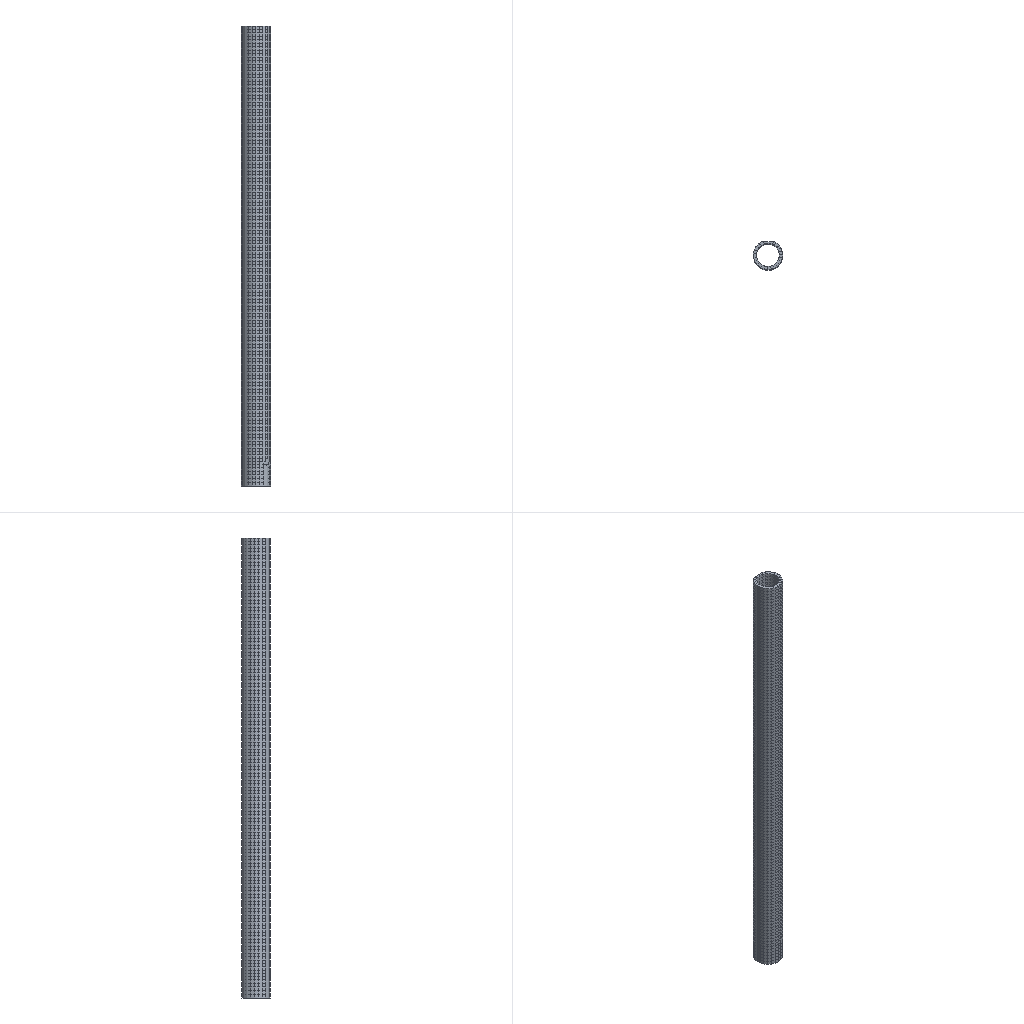Simulation study | abaqus
Set-up summary:
category,name,step,type,value,unit,region
solver,abaqus,,Abaqus/CAE 2024
units,mm-N-s-tonne (MPa),,inferred,E=210000 density=
analysis,Step-4,,static,time_period=10
mesh,nodes,,,6433
mesh,elements,,,3192
element_type,C3D8R,,,3192
material,Material-1,,E,210000
material,Material-1,,nu,0.3
material,Material-1,,yield,380
material,Material-1,,cte,1.3e-05
material,Material-1,,behaviors,plastic; expansion
section,Material-1,,solid section,,,Set-1
load,Load-2,Step-4,pressure,30,,Surf-6
load,Load-4,Step-4,concentrated force,"1000 [dir=(0, 1, 0)]",,Set-13
bc,BC-1,initial,fixed,"[dofs=rx,ry,rz,x,y,z n=6]",,Set-5
bc,BC-2,Step-4,displacement,-0.5 [dofs=rx],,_PickedSet34
bc,BC-2,Step-4,fixed,"[dofs=ry,rz n=2]",,_PickedSet34
constraint,coupling,,,1
Abaqus input file, long lists of numbers shortened:
*Heading
** Job name: deck Model name: Model-1-3
** Generated by: Abaqus/CAE 2024
*Preprint, echo=NO, model=NO, history=NO, contact=NO
**
** PARTS
**
*Part, name=Part-10
*Node
      1,           0.,          58.,         120.
      2,           0.,          50.,         120.
** (6430 more lines like these left out)
*Element, type=C3D8R
   1,    1,    2,   33,    5,   54,  301,  973,  549
   2,    5,   33,   34,   47,  549,  973,  974, 2471
** (3190 more lines like these left out)
*Nset, nset=Set-1, generate
    1,  6432,     1
*Elset, elset=Set-1, generate
    1,  3192,     1
** Section: Section-1
*Solid Section, elset=Set-1, material=Material-1
,
*End Part
**
**
** ASSEMBLY
**
*Assembly, name=Assembly
**
*Instance, name=Part-10-1, part=Part-10
*End Instance
**
*Node
      1,           0., -3.91886993e-15,        2000.
*Nset, nset=Set-5, instance=Part-10-1
  22,  23,  24,  25,  26,  30,  31,  32, 906, 907, 908, 909, 910, 911, 912, 913
 914, 915, 916, 917, 918, 919, 920, 921, 922, 923, 924, 952, 953, 954, 955, 956
** (1 more lines like these left out)
*Elset, elset=Set-5, instance=Part-10-1
 3078, 3079, 3080, 3081, 3082, 3083, 3084, 3085, 3086, 3087, 3088, 3180, 3181, 3182, 3183, 3184
 3185, 3186, 3187, 3188, 3189, 3190, 3191, 3192
*Nset, nset=Set-13
 1,
*Nset, nset=m_Set-12
 1,
*Nset, nset=s_Set-8, instance=Part-10-1
   8,   9,  10,  11,  12,  13,  14,  16, 674, 675, 676, 677, 678, 679, 680, 681
 682, 683, 684, 685, 686, 687, 688, 689, 690, 691, 692, 693, 694, 838, 839, 840
** (1 more lines like these left out)
*Elset, elset=s_Set-8, instance=Part-10-1
 1613, 1614, 1615, 1616, 1617, 1618, 1619, 1620, 1621, 1622, 1623, 1624, 1625, 2990, 2991, 2992
 2993, 2994, 2995, 2996, 2997, 2998, 2999, 3000
*Nset, nset=_PickedSet34, internal
 1,
*Elset, elset=_Surf-2_S3, internal, instance=Part-10-1, generate
 3001,  3088,     1
*Elset, elset=_Surf-2_S5, internal, instance=Part-10-1, generate
 3089,  3192,     1
*Elset, elset=_Surf-2_S4, internal, instance=Part-10-1, generate
    1,  1625,     1
*Elset, elset=_Surf-2_S6, internal, instance=Part-10-1, generate
 1626,  3000,     1
*Surface, type=ELEMENT, name=Surf-2
_Surf-2_S3, S3
_Surf-2_S5, S5
_Surf-2_S4, S4
_Surf-2_S6, S6
*Elset, elset=_Surf-5_S5, internal, instance=Part-10-1
 3035, 3036, 3037, 3038, 3039, 3040, 3041, 3042, 3043, 3044, 3046, 3047, 3048, 3049, 3050, 3051
 3052, 3053, 3054, 3055, 3057, 3058, 3059, 3060, 3061, 3062, 3063, 3064, 3065, 3066, 3068, 3069
** (2 more lines like these left out)
*Elset, elset=_Surf-5_S3, internal, instance=Part-10-1
 3129, 3130, 3131, 3132, 3133, 3134, 3135, 3136, 3137, 3138, 3139, 3140, 3142, 3143, 3144, 3145
 3146, 3147, 3148, 3149, 3150, 3151, 3152, 3153, 3155, 3156, 3157, 3158, 3159, 3160, 3161, 3162
** (2 more lines like these left out)
*Elset, elset=_Surf-5_S4, internal, instance=Part-10-1
 1627, 1628, 1629, 1630, 1631, 1632, 1633, 1634, 1635, 1636, 1638, 1639, 1640, 1641, 1642, 1643
 1644, 1645, 1646, 1647, 1649, 1650, 1651, 1652, 1653, 1654, 1655, 1656, 1657, 1658, 1660, 1661
** (77 more lines like these left out)
*Elset, elset=_Surf-5_S6, internal, instance=Part-10-1
    2,    3,    4,    5,    6,    7,    8,    9,   10,   11,   12,   13,   15,   16,   17,   18
   19,   20,   21,   22,   23,   24,   25,   26,   28,   29,   30,   31,   32,   33,   34,   35
** (92 more lines like these left out)
*Surface, type=ELEMENT, name=Surf-5
_Surf-5_S5, S5
_Surf-5_S3, S3
_Surf-5_S4, S4
_Surf-5_S6, S6
*Elset, elset=_Surf-6_S3, internal, instance=Part-10-1, generate
 3089,  3192,     1
*Elset, elset=_Surf-6_S5, internal, instance=Part-10-1, generate
 3001,  3088,     1
*Elset, elset=_Surf-6_S4, internal, instance=Part-10-1, generate
 1626,  3000,     1
*Elset, elset=_Surf-6_S6, internal, instance=Part-10-1, generate
    1,  1625,     1
*Surface, type=ELEMENT, name=Surf-6
_Surf-6_S3, S3
_Surf-6_S5, S5
_Surf-6_S4, S4
_Surf-6_S6, S6
*Elset, elset=_m_Surf-3_S2, internal, instance=Part-10-1
 1613, 1614, 1615, 1616, 1617, 1618, 1619, 1620, 1621, 1622, 1623, 1624, 1625, 2990, 2991, 2992
 2993, 2994, 2995, 2996, 2997, 2998, 2999, 3000
*Surface, type=ELEMENT, name=m_Surf-3
_m_Surf-3_S2, S2
*Elset, elset=_s_Surf-4_S2, internal, instance=Part-10-1
 1613, 1614, 1615, 1616, 1617, 1618, 1619, 1620, 1621, 1622, 1623, 1624, 1625, 2990, 2991, 2992
 2993, 2994, 2995, 2996, 2997, 2998, 2999, 3000
*Surface, type=ELEMENT, name=s_Surf-4
_s_Surf-4_S2, S2
** Constraint: Constraint-3
*Coupling, constraint name=Constraint-3, ref node=m_Set-12, surface=s_Surf-4
*Kinematic
*End Assembly
**
** MATERIALS
**
*Material, name=Material-1
*Elastic
210000., 0.3
*Expansion
 1.3e-05,
*Plastic
380.,  0.
600., 0.2
**
** BOUNDARY CONDITIONS
**
** Name: BC-1 Type: Displacement/Rotation
*Boundary
Set-5, 1, 1
Set-5, 2, 2
Set-5, 3, 3
Set-5, 4, 4
Set-5, 5, 5
Set-5, 6, 6
** ----------------------------------------------------------------
**
** STEP: Step-4
**
*Step, name=Step-4, nlgeom=NO, inc=1000
*Static
1., 10., 0.0001, 1.
**
** BOUNDARY CONDITIONS
**
** Name: BC-2 Type: Displacement/Rotation
*Boundary
_PickedSet34, 4, 4, -0.5
_PickedSet34, 5, 5
_PickedSet34, 6, 6
**
** LOADS
**
** Name: Load-2   Type: Pressure
*Dsload
Surf-6, P, 30.
** Name: Load-4   Type: Concentrated force
*Cload
Set-13, 2, 1000.
**
** OUTPUT REQUESTS
**
*Restart, write, frequency=0
**
** FIELD OUTPUT: F-Output-2
**
*Output, field
*Node Output
CF, RF, RM, RT, TF, U, UR, UT
V, VF, VR, VT
*Element Output, directions=YES
ALPHA, ALPHAN, BF, CENTMAG, CENTRIFMAG, CORIOMAG, CS11, CTSHR, E, EE, EEQUT, ER, ESF1, GRAV, HP, IE
LE, LODE, MISES, MISESMAX, MISESONLY, NE, NFORC, NFORCSO, P, PE, PEEQ, PEEQMAX, PEEQT, PEMAG, PEQC, PRESSONLY
PS, ROTAMAG, S, SALPHA, SE, SEE, SEP, SEPE, SEQUT, SF, SPE, SQEQ, SSAVG, TE, TEEQ, TEVOL
THE, TRIAX, TRNOR, TRSHR, TSHR, VE, VEEQ, VS, YIELDPOT
**
** HISTORY OUTPUT: H-Output-2
**
*Output, history
*Element Output
IRA1, IRA2, IRA3, IRAR1, IRAR2, IRAR3, IRF1, IRF2, IRF3, IRM1, IRM2, IRM3
*End Step
Results summary:
result,odb.job_status,,,JOB_STATUS_COMPLETED_SUCCESSFULLY,"consistent, unstated (Abaqus has no unit system)"
result,steps[0].procedure,Step-4,,*STATIC,"consistent, unstated (Abaqus has no unit system)"
result,steps[0].time_period,Step-4,,10,"consistent, unstated (Abaqus has no unit system)"
result,steps[0].n_frames,Step-4,,11,"consistent, unstated (Abaqus has no unit system)"
result,steps[0].last_frame.id,Step-4,,10,"consistent, unstated (Abaqus has no unit system)"
result,steps[0].last_frame.value,Step-4,,10,"consistent, unstated (Abaqus has no unit system)"
result,steps[0].last_frame.description,Step-4,,Increment     10: Step Time =    10.00,"consistent, unstated (Abaqus has no unit system)"
result,steps[0].completed,Step-4,,True,"consistent, unstated (Abaqus has no unit system)"
result,steps[0].max_U_magnitude,Step-4,,555.581,"consistent, unstated (Abaqus has no unit system)"
result,steps[0].max_S_mises,Step-4,,408.187,"consistent, unstated (Abaqus has no unit system)"
result,steps[0].RF_sum[1],Step-4,,0.0001373,"consistent, unstated (Abaqus has no unit system)"
result,steps[0].RF_sum[2],Step-4,,-1000,"consistent, unstated (Abaqus has no unit system)"
result,steps[0].RF_sum[3],Step-4,,-325.031,"consistent, unstated (Abaqus has no unit system)"